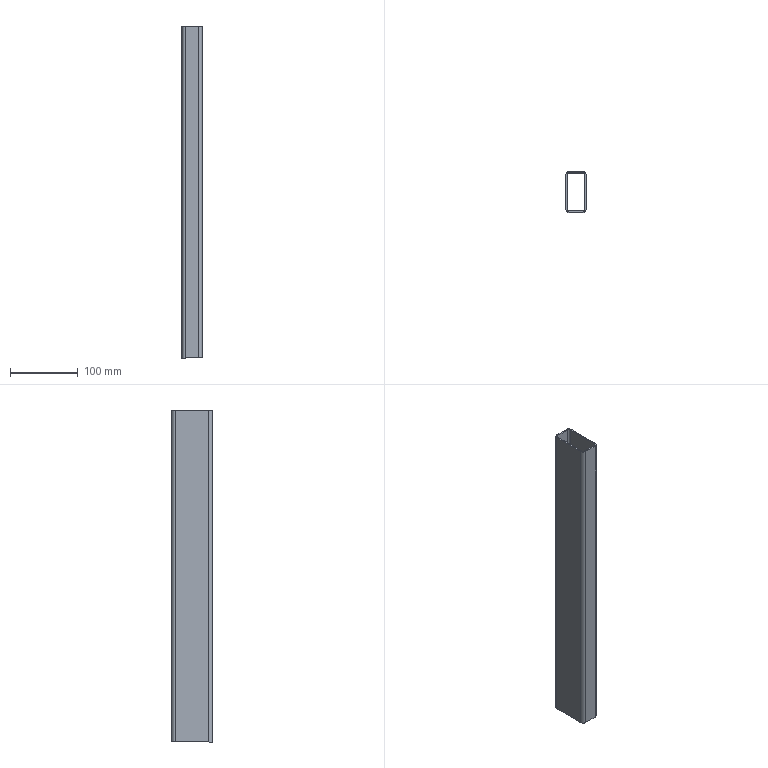Part | SolidWorks | features BaseBody 1 | 1 solid | 18 faces | box 30 x 60 x 490 mm | volume 161830 mm3 | plane 10 | cylinder 8 | commonest cylinder face diameters 6 x4 10 x4
STEP:
#1=CARTESIAN_POINT('',(10.,28.,490.));
#2=VERTEX_POINT('',#1);
#3=CARTESIAN_POINT('',(-10.,28.,490.));
#4=VERTEX_POINT('',#3);
#5=CARTESIAN_POINT('',(-5.,28.,490.));
#6=DIRECTION('',(-1.,0.,0.));
#7=VECTOR('',#6,1000.);
#8=LINE('',#5,#7);
#9=EDGE_CURVE('',#2,#4,#8,.T.);
#10=ORIENTED_EDGE('',*,*,#9,.F.);
#11=CARTESIAN_POINT('',(13.,25.,490.));
#12=VERTEX_POINT('',#11);
#13=CARTESIAN_POINT('',(10.,25.,490.));
#14=DIRECTION('',(0.,0.,1.));
#15=DIRECTION('',(-1.,0.,0.));
#16=AXIS2_PLACEMENT_3D('',#13,#14,#15);
#17=CIRCLE('',#16,3.);
#18=EDGE_CURVE('',#12,#2,#17,.T.);
#19=ORIENTED_EDGE('',*,*,#18,.F.);
#20=CARTESIAN_POINT('',(13.,-25.,490.));
#21=VERTEX_POINT('',#20);
#22=CARTESIAN_POINT('',(13.,12.5,490.));
#23=DIRECTION('',(0.,1.,0.));
#24=VECTOR('',#23,1000.);
#25=LINE('',#22,#24);
#26=EDGE_CURVE('',#21,#12,#25,.T.);
#27=ORIENTED_EDGE('',*,*,#26,.F.);
#28=CARTESIAN_POINT('',(10.,-28.,490.));
#29=VERTEX_POINT('',#28);
#30=CARTESIAN_POINT('',(10.,-25.,490.));
#31=DIRECTION('',(0.,0.,1.));
#32=DIRECTION('',(0.,1.,0.));
#33=AXIS2_PLACEMENT_3D('',#30,#31,#32);
#34=CIRCLE('',#33,3.);
#35=EDGE_CURVE('',#29,#21,#34,.T.);
#36=ORIENTED_EDGE('',*,*,#35,.F.);
#37=CARTESIAN_POINT('',(-10.,-28.,490.));
#38=VERTEX_POINT('',#37);
#39=CARTESIAN_POINT('',(5.,-28.,490.));
#40=DIRECTION('',(1.,0.,0.));
#41=VECTOR('',#40,1000.);
#42=LINE('',#39,#41);
#43=EDGE_CURVE('',#38,#29,#42,.T.);
#44=ORIENTED_EDGE('',*,*,#43,.F.);
#45=CARTESIAN_POINT('',(-13.,-25.,490.));
#46=VERTEX_POINT('',#45);
#47=CARTESIAN_POINT('',(-10.,-25.,490.));
#48=DIRECTION('',(0.,0.,1.));
#49=DIRECTION('',(1.,0.,0.));
#50=AXIS2_PLACEMENT_3D('',#47,#48,#49);
#51=CIRCLE('',#50,3.);
#52=EDGE_CURVE('',#46,#38,#51,.T.);
#53=ORIENTED_EDGE('',*,*,#52,.F.);
#54=CARTESIAN_POINT('',(-13.,25.,490.));
#55=VERTEX_POINT('',#54);
#56=CARTESIAN_POINT('',(-13.,-12.5,490.));
#57=DIRECTION('',(0.,-1.,0.));
#58=VECTOR('',#57,1000.);
#59=LINE('',#56,#58);
#60=EDGE_CURVE('',#55,#46,#59,.T.);
#61=ORIENTED_EDGE('',*,*,#60,.F.);
#62=CARTESIAN_POINT('',(-10.,25.,490.));
#63=DIRECTION('',(0.,0.,1.));
#64=DIRECTION('',(0.,-1.,0.));
#65=AXIS2_PLACEMENT_3D('',#62,#63,#64);
#66=CIRCLE('',#65,3.);
#67=EDGE_CURVE('',#4,#55,#66,.T.);
#68=ORIENTED_EDGE('',*,*,#67,.F.);
#69=EDGE_LOOP('',(#10,#19,#27,#36,#44,#53,#61,#68));
#70=FACE_BOUND('',#69,.T.);
#71=CARTESIAN_POINT('',(-15.,-25.,490.));
#72=VERTEX_POINT('',#71);
#73=CARTESIAN_POINT('',(-15.,25.,490.));
#74=VERTEX_POINT('',#73);
#75=CARTESIAN_POINT('',(-15.,-12.5,490.));
#76=DIRECTION('',(0.,1.,0.));
#77=VECTOR('',#76,1000.);
#78=LINE('',#75,#77);
#79=EDGE_CURVE('',#72,#74,#78,.T.);
#80=ORIENTED_EDGE('',*,*,#79,.F.);
#81=CARTESIAN_POINT('',(-10.,-30.,490.));
#82=VERTEX_POINT('',#81);
#83=CARTESIAN_POINT('',(-10.,-25.,490.));
#84=DIRECTION('',(0.,0.,-1.));
#85=DIRECTION('',(1.,0.,0.));
#86=AXIS2_PLACEMENT_3D('',#83,#84,#85);
#87=CIRCLE('',#86,5.);
#88=EDGE_CURVE('',#82,#72,#87,.T.);
#89=ORIENTED_EDGE('',*,*,#88,.F.);
#90=CARTESIAN_POINT('',(10.,-30.,490.));
#91=VERTEX_POINT('',#90);
#92=CARTESIAN_POINT('',(5.,-30.,490.));
#93=DIRECTION('',(-1.,0.,0.));
#94=VECTOR('',#93,1000.);
#95=LINE('',#92,#94);
#96=EDGE_CURVE('',#91,#82,#95,.T.);
#97=ORIENTED_EDGE('',*,*,#96,.F.);
#98=CARTESIAN_POINT('',(15.,-25.,490.));
#99=VERTEX_POINT('',#98);
#100=CARTESIAN_POINT('',(10.,-25.,490.));
#101=DIRECTION('',(0.,0.,-1.));
#102=DIRECTION('',(0.,1.,0.));
#103=AXIS2_PLACEMENT_3D('',#100,#101,#102);
#104=CIRCLE('',#103,5.);
#105=EDGE_CURVE('',#99,#91,#104,.T.);
#106=ORIENTED_EDGE('',*,*,#105,.F.);
#107=CARTESIAN_POINT('',(15.,25.,490.));
#108=VERTEX_POINT('',#107);
#109=CARTESIAN_POINT('',(15.,12.5,490.));
#110=DIRECTION('',(0.,-1.,0.));
#111=VECTOR('',#110,1000.);
#112=LINE('',#109,#111);
#113=EDGE_CURVE('',#108,#99,#112,.T.);
#114=ORIENTED_EDGE('',*,*,#113,.F.);
#115=CARTESIAN_POINT('',(10.,30.,490.));
#116=VERTEX_POINT('',#115);
#117=CARTESIAN_POINT('',(10.,25.,490.));
#118=DIRECTION('',(0.,0.,-1.));
#119=DIRECTION('',(-1.,0.,0.));
#120=AXIS2_PLACEMENT_3D('',#117,#118,#119);
#121=CIRCLE('',#120,5.);
#122=EDGE_CURVE('',#116,#108,#121,.T.);
#123=ORIENTED_EDGE('',*,*,#122,.F.);
#124=CARTESIAN_POINT('',(-10.,30.,490.));
#125=VERTEX_POINT('',#124);
#126=CARTESIAN_POINT('',(-5.,30.,490.));
#127=DIRECTION('',(1.,0.,0.));
#128=VECTOR('',#127,1000.);
#129=LINE('',#126,#128);
#130=EDGE_CURVE('',#125,#116,#129,.T.);
#131=ORIENTED_EDGE('',*,*,#130,.F.);
#132=CARTESIAN_POINT('',(-10.,25.,490.));
#133=DIRECTION('',(0.,0.,-1.));
#134=DIRECTION('',(0.,-1.,0.));
#135=AXIS2_PLACEMENT_3D('',#132,#133,#134);
#136=CIRCLE('',#135,5.);
#137=EDGE_CURVE('',#74,#125,#136,.T.);
#138=ORIENTED_EDGE('',*,*,#137,.F.);
#139=EDGE_LOOP('',(#80,#89,#97,#106,#114,#123,#131,#138));
#140=FACE_OUTER_BOUND('',#139,.T.);
#141=CARTESIAN_POINT('',(0.,0.,490.));
#142=DIRECTION('',(0.,0.,1.));
#143=DIRECTION('',(1.,0.,0.));
#144=AXIS2_PLACEMENT_3D('',#141,#142,#143);
#145=PLANE('',#144);
#146=ADVANCED_FACE('',(#70,#140),#145,.T.);
#147=CARTESIAN_POINT('',(10.,28.,0.));
#148=VERTEX_POINT('',#147);
#149=CARTESIAN_POINT('',(-10.,28.,0.));
#150=VERTEX_POINT('',#149);
#151=CARTESIAN_POINT('',(-5.,28.,0.));
#152=DIRECTION('',(-1.,0.,0.));
#153=VECTOR('',#152,1000.);
#154=LINE('',#151,#153);
#155=EDGE_CURVE('',#148,#150,#154,.T.);
#156=ORIENTED_EDGE('',*,*,#155,.T.);
#157=CARTESIAN_POINT('',(-13.,25.,0.));
#158=VERTEX_POINT('',#157);
#159=CARTESIAN_POINT('',(-10.,25.,0.));
#160=DIRECTION('',(0.,0.,1.));
#161=DIRECTION('',(0.,-1.,0.));
#162=AXIS2_PLACEMENT_3D('',#159,#160,#161);
#163=CIRCLE('',#162,3.);
#164=EDGE_CURVE('',#150,#158,#163,.T.);
#165=ORIENTED_EDGE('',*,*,#164,.T.);
#166=CARTESIAN_POINT('',(-13.,-25.,0.));
#167=VERTEX_POINT('',#166);
#168=CARTESIAN_POINT('',(-13.,-12.5,0.));
#169=DIRECTION('',(0.,-1.,0.));
#170=VECTOR('',#169,1000.);
#171=LINE('',#168,#170);
#172=EDGE_CURVE('',#158,#167,#171,.T.);
#173=ORIENTED_EDGE('',*,*,#172,.T.);
#174=CARTESIAN_POINT('',(-10.,-28.,0.));
#175=VERTEX_POINT('',#174);
#176=CARTESIAN_POINT('',(-10.,-25.,0.));
#177=DIRECTION('',(0.,0.,1.));
#178=DIRECTION('',(1.,0.,0.));
#179=AXIS2_PLACEMENT_3D('',#176,#177,#178);
#180=CIRCLE('',#179,3.);
#181=EDGE_CURVE('',#167,#175,#180,.T.);
#182=ORIENTED_EDGE('',*,*,#181,.T.);
#183=CARTESIAN_POINT('',(10.,-28.,0.));
#184=VERTEX_POINT('',#183);
#185=CARTESIAN_POINT('',(5.,-28.,0.));
#186=DIRECTION('',(1.,0.,0.));
#187=VECTOR('',#186,1000.);
#188=LINE('',#185,#187);
#189=EDGE_CURVE('',#175,#184,#188,.T.);
#190=ORIENTED_EDGE('',*,*,#189,.T.);
#191=CARTESIAN_POINT('',(13.,-25.,0.));
#192=VERTEX_POINT('',#191);
#193=CARTESIAN_POINT('',(10.,-25.,0.));
#194=DIRECTION('',(0.,0.,1.));
#195=DIRECTION('',(0.,1.,0.));
#196=AXIS2_PLACEMENT_3D('',#193,#194,#195);
#197=CIRCLE('',#196,3.);
#198=EDGE_CURVE('',#184,#192,#197,.T.);
#199=ORIENTED_EDGE('',*,*,#198,.T.);
#200=CARTESIAN_POINT('',(13.,25.,0.));
#201=VERTEX_POINT('',#200);
#202=CARTESIAN_POINT('',(13.,12.5,0.));
#203=DIRECTION('',(0.,1.,0.));
#204=VECTOR('',#203,1000.);
#205=LINE('',#202,#204);
#206=EDGE_CURVE('',#192,#201,#205,.T.);
#207=ORIENTED_EDGE('',*,*,#206,.T.);
#208=CARTESIAN_POINT('',(10.,25.,0.));
#209=DIRECTION('',(0.,0.,1.));
#210=DIRECTION('',(-1.,0.,0.));
#211=AXIS2_PLACEMENT_3D('',#208,#209,#210);
#212=CIRCLE('',#211,3.);
#213=EDGE_CURVE('',#201,#148,#212,.T.);
#214=ORIENTED_EDGE('',*,*,#213,.T.);
#215=EDGE_LOOP('',(#156,#165,#173,#182,#190,#199,#207,#214));
#216=FACE_BOUND('',#215,.T.);
#217=CARTESIAN_POINT('',(-15.,-25.,0.));
#218=VERTEX_POINT('',#217);
#219=CARTESIAN_POINT('',(-15.,25.,0.));
#220=VERTEX_POINT('',#219);
#221=CARTESIAN_POINT('',(-15.,-12.5,0.));
#222=DIRECTION('',(0.,1.,0.));
#223=VECTOR('',#222,1000.);
#224=LINE('',#221,#223);
#225=EDGE_CURVE('',#218,#220,#224,.T.);
#226=ORIENTED_EDGE('',*,*,#225,.T.);
#227=CARTESIAN_POINT('',(-10.,30.,0.));
#228=VERTEX_POINT('',#227);
#229=CARTESIAN_POINT('',(-10.,25.,0.));
#230=DIRECTION('',(0.,0.,-1.));
#231=DIRECTION('',(0.,-1.,0.));
#232=AXIS2_PLACEMENT_3D('',#229,#230,#231);
#233=CIRCLE('',#232,5.);
#234=EDGE_CURVE('',#220,#228,#233,.T.);
#235=ORIENTED_EDGE('',*,*,#234,.T.);
#236=CARTESIAN_POINT('',(10.,30.,0.));
#237=VERTEX_POINT('',#236);
#238=CARTESIAN_POINT('',(-5.,30.,0.));
#239=DIRECTION('',(1.,0.,0.));
#240=VECTOR('',#239,1000.);
#241=LINE('',#238,#240);
#242=EDGE_CURVE('',#228,#237,#241,.T.);
#243=ORIENTED_EDGE('',*,*,#242,.T.);
#244=CARTESIAN_POINT('',(15.,25.,0.));
#245=VERTEX_POINT('',#244);
#246=CARTESIAN_POINT('',(10.,25.,0.));
#247=DIRECTION('',(0.,0.,-1.));
#248=DIRECTION('',(-1.,0.,0.));
#249=AXIS2_PLACEMENT_3D('',#246,#247,#248);
#250=CIRCLE('',#249,5.);
#251=EDGE_CURVE('',#237,#245,#250,.T.);
#252=ORIENTED_EDGE('',*,*,#251,.T.);
#253=CARTESIAN_POINT('',(15.,-25.,0.));
#254=VERTEX_POINT('',#253);
#255=CARTESIAN_POINT('',(15.,12.5,0.));
#256=DIRECTION('',(0.,-1.,0.));
#257=VECTOR('',#256,1000.);
#258=LINE('',#255,#257);
#259=EDGE_CURVE('',#245,#254,#258,.T.);
#260=ORIENTED_EDGE('',*,*,#259,.T.);
#261=CARTESIAN_POINT('',(10.,-30.,0.));
#262=VERTEX_POINT('',#261);
#263=CARTESIAN_POINT('',(10.,-25.,0.));
#264=DIRECTION('',(0.,0.,-1.));
#265=DIRECTION('',(0.,1.,0.));
#266=AXIS2_PLACEMENT_3D('',#263,#264,#265);
#267=CIRCLE('',#266,5.);
#268=EDGE_CURVE('',#254,#262,#267,.T.);
#269=ORIENTED_EDGE('',*,*,#268,.T.);
#270=CARTESIAN_POINT('',(-10.,-30.,0.));
#271=VERTEX_POINT('',#270);
#272=CARTESIAN_POINT('',(5.,-30.,0.));
#273=DIRECTION('',(-1.,0.,0.));
#274=VECTOR('',#273,1000.);
#275=LINE('',#272,#274);
#276=EDGE_CURVE('',#262,#271,#275,.T.);
#277=ORIENTED_EDGE('',*,*,#276,.T.);
#278=CARTESIAN_POINT('',(-10.,-25.,0.));
#279=DIRECTION('',(0.,0.,-1.));
#280=DIRECTION('',(1.,0.,0.));
#281=AXIS2_PLACEMENT_3D('',#278,#279,#280);
#282=CIRCLE('',#281,5.);
#283=EDGE_CURVE('',#271,#218,#282,.T.);
#284=ORIENTED_EDGE('',*,*,#283,.T.);
#285=EDGE_LOOP('',(#226,#235,#243,#252,#260,#269,#277,#284));
#286=FACE_OUTER_BOUND('',#285,.T.);
#287=CARTESIAN_POINT('',(0.,0.,0.));
#288=DIRECTION('',(0.,0.,1.));
#289=DIRECTION('',(1.,0.,0.));
#290=AXIS2_PLACEMENT_3D('',#287,#288,#289);
#291=PLANE('',#290);
#292=ADVANCED_FACE('',(#216,#286),#291,.F.);
#293=ORIENTED_EDGE('',*,*,#122,.T.);
#294=CARTESIAN_POINT('',(15.,25.,0.));
#295=DIRECTION('',(0.,0.,1.));
#296=VECTOR('',#295,1000.);
#297=LINE('',#294,#296);
#298=EDGE_CURVE('',#245,#108,#297,.T.);
#299=ORIENTED_EDGE('',*,*,#298,.F.);
#300=ORIENTED_EDGE('',*,*,#251,.F.);
#301=CARTESIAN_POINT('',(10.,30.,0.));
#302=DIRECTION('',(0.,0.,1.));
#303=VECTOR('',#302,1000.);
#304=LINE('',#301,#303);
#305=EDGE_CURVE('',#237,#116,#304,.T.);
#306=ORIENTED_EDGE('',*,*,#305,.T.);
#307=EDGE_LOOP('',(#293,#299,#300,#306));
#308=FACE_OUTER_BOUND('',#307,.T.);
#309=CARTESIAN_POINT('',(10.,25.,0.));
#310=DIRECTION('',(0.,0.,1.));
#311=DIRECTION('',(-1.,0.,0.));
#312=AXIS2_PLACEMENT_3D('',#309,#310,#311);
#313=CYLINDRICAL_SURFACE('',#312,5.);
#314=ADVANCED_FACE('',(#308),#313,.T.);
#315=ORIENTED_EDGE('',*,*,#130,.T.);
#316=ORIENTED_EDGE('',*,*,#305,.F.);
#317=ORIENTED_EDGE('',*,*,#242,.F.);
#318=CARTESIAN_POINT('',(-10.,30.,0.));
#319=DIRECTION('',(0.,0.,1.));
#320=VECTOR('',#319,1000.);
#321=LINE('',#318,#320);
#322=EDGE_CURVE('',#228,#125,#321,.T.);
#323=ORIENTED_EDGE('',*,*,#322,.T.);
#324=EDGE_LOOP('',(#315,#316,#317,#323));
#325=FACE_OUTER_BOUND('',#324,.T.);
#326=CARTESIAN_POINT('',(-10.,30.,0.));
#327=DIRECTION('',(0.,1.,0.));
#328=DIRECTION('',(1.,0.,0.));
#329=AXIS2_PLACEMENT_3D('',#326,#327,#328);
#330=PLANE('',#329);
#331=ADVANCED_FACE('',(#325),#330,.T.);
#332=ORIENTED_EDGE('',*,*,#137,.T.);
#333=ORIENTED_EDGE('',*,*,#322,.F.);
#334=ORIENTED_EDGE('',*,*,#234,.F.);
#335=CARTESIAN_POINT('',(-15.,25.,0.));
#336=DIRECTION('',(0.,0.,1.));
#337=VECTOR('',#336,1000.);
#338=LINE('',#335,#337);
#339=EDGE_CURVE('',#220,#74,#338,.T.);
#340=ORIENTED_EDGE('',*,*,#339,.T.);
#341=EDGE_LOOP('',(#332,#333,#334,#340));
#342=FACE_OUTER_BOUND('',#341,.T.);
#343=CARTESIAN_POINT('',(-10.,25.,0.));
#344=DIRECTION('',(0.,0.,1.));
#345=DIRECTION('',(0.,-1.,0.));
#346=AXIS2_PLACEMENT_3D('',#343,#344,#345);
#347=CYLINDRICAL_SURFACE('',#346,5.);
#348=ADVANCED_FACE('',(#342),#347,.T.);
#349=ORIENTED_EDGE('',*,*,#79,.T.);
#350=ORIENTED_EDGE('',*,*,#339,.F.);
#351=ORIENTED_EDGE('',*,*,#225,.F.);
#352=CARTESIAN_POINT('',(-15.,-25.,0.));
#353=DIRECTION('',(0.,0.,1.));
#354=VECTOR('',#353,1000.);
#355=LINE('',#352,#354);
#356=EDGE_CURVE('',#218,#72,#355,.T.);
#357=ORIENTED_EDGE('',*,*,#356,.T.);
#358=EDGE_LOOP('',(#349,#350,#351,#357));
#359=FACE_OUTER_BOUND('',#358,.T.);
#360=CARTESIAN_POINT('',(-15.,-25.,0.));
#361=DIRECTION('',(-1.,0.,0.));
#362=DIRECTION('',(0.,1.,0.));
#363=AXIS2_PLACEMENT_3D('',#360,#361,#362);
#364=PLANE('',#363);
#365=ADVANCED_FACE('',(#359),#364,.T.);
#366=ORIENTED_EDGE('',*,*,#67,.T.);
#367=CARTESIAN_POINT('',(-13.,25.,0.));
#368=DIRECTION('',(0.,0.,1.));
#369=VECTOR('',#368,1000.);
#370=LINE('',#367,#369);
#371=EDGE_CURVE('',#158,#55,#370,.T.);
#372=ORIENTED_EDGE('',*,*,#371,.F.);
#373=ORIENTED_EDGE('',*,*,#164,.F.);
#374=CARTESIAN_POINT('',(-10.,28.,0.));
#375=DIRECTION('',(0.,0.,1.));
#376=VECTOR('',#375,1000.);
#377=LINE('',#374,#376);
#378=EDGE_CURVE('',#150,#4,#377,.T.);
#379=ORIENTED_EDGE('',*,*,#378,.T.);
#380=EDGE_LOOP('',(#366,#372,#373,#379));
#381=FACE_OUTER_BOUND('',#380,.T.);
#382=CARTESIAN_POINT('',(-10.,25.,0.));
#383=DIRECTION('',(0.,0.,1.));
#384=DIRECTION('',(0.,-1.,0.));
#385=AXIS2_PLACEMENT_3D('',#382,#383,#384);
#386=CYLINDRICAL_SURFACE('',#385,3.);
#387=ADVANCED_FACE('',(#381),#386,.F.);
#388=ORIENTED_EDGE('',*,*,#60,.T.);
#389=CARTESIAN_POINT('',(-13.,-25.,0.));
#390=DIRECTION('',(0.,0.,1.));
#391=VECTOR('',#390,1000.);
#392=LINE('',#389,#391);
#393=EDGE_CURVE('',#167,#46,#392,.T.);
#394=ORIENTED_EDGE('',*,*,#393,.F.);
#395=ORIENTED_EDGE('',*,*,#172,.F.);
#396=ORIENTED_EDGE('',*,*,#371,.T.);
#397=EDGE_LOOP('',(#388,#394,#395,#396));
#398=FACE_OUTER_BOUND('',#397,.T.);
#399=CARTESIAN_POINT('',(-13.,-25.,0.));
#400=DIRECTION('',(-1.,0.,0.));
#401=DIRECTION('',(0.,1.,0.));
#402=AXIS2_PLACEMENT_3D('',#399,#400,#401);
#403=PLANE('',#402);
#404=ADVANCED_FACE('',(#398),#403,.F.);
#405=ORIENTED_EDGE('',*,*,#52,.T.);
#406=CARTESIAN_POINT('',(-10.,-28.,0.));
#407=DIRECTION('',(0.,0.,1.));
#408=VECTOR('',#407,1000.);
#409=LINE('',#406,#408);
#410=EDGE_CURVE('',#175,#38,#409,.T.);
#411=ORIENTED_EDGE('',*,*,#410,.F.);
#412=ORIENTED_EDGE('',*,*,#181,.F.);
#413=ORIENTED_EDGE('',*,*,#393,.T.);
#414=EDGE_LOOP('',(#405,#411,#412,#413));
#415=FACE_OUTER_BOUND('',#414,.T.);
#416=CARTESIAN_POINT('',(-10.,-25.,0.));
#417=DIRECTION('',(0.,0.,1.));
#418=DIRECTION('',(1.,0.,0.));
#419=AXIS2_PLACEMENT_3D('',#416,#417,#418);
#420=CYLINDRICAL_SURFACE('',#419,3.);
#421=ADVANCED_FACE('',(#415),#420,.F.);
#422=ORIENTED_EDGE('',*,*,#9,.T.);
#423=ORIENTED_EDGE('',*,*,#378,.F.);
#424=ORIENTED_EDGE('',*,*,#155,.F.);
#425=CARTESIAN_POINT('',(10.,28.,0.));
#426=DIRECTION('',(0.,0.,1.));
#427=VECTOR('',#426,1000.);
#428=LINE('',#425,#427);
#429=EDGE_CURVE('',#148,#2,#428,.T.);
#430=ORIENTED_EDGE('',*,*,#429,.T.);
#431=EDGE_LOOP('',(#422,#423,#424,#430));
#432=FACE_OUTER_BOUND('',#431,.T.);
#433=CARTESIAN_POINT('',(-10.,28.,0.));
#434=DIRECTION('',(0.,1.,0.));
#435=DIRECTION('',(1.,0.,0.));
#436=AXIS2_PLACEMENT_3D('',#433,#434,#435);
#437=PLANE('',#436);
#438=ADVANCED_FACE('',(#432),#437,.F.);
#439=ORIENTED_EDGE('',*,*,#88,.T.);
#440=ORIENTED_EDGE('',*,*,#356,.F.);
#441=ORIENTED_EDGE('',*,*,#283,.F.);
#442=CARTESIAN_POINT('',(-10.,-30.,0.));
#443=DIRECTION('',(0.,0.,1.));
#444=VECTOR('',#443,1000.);
#445=LINE('',#442,#444);
#446=EDGE_CURVE('',#271,#82,#445,.T.);
#447=ORIENTED_EDGE('',*,*,#446,.T.);
#448=EDGE_LOOP('',(#439,#440,#441,#447));
#449=FACE_OUTER_BOUND('',#448,.T.);
#450=CARTESIAN_POINT('',(-10.,-25.,0.));
#451=DIRECTION('',(0.,0.,1.));
#452=DIRECTION('',(1.,0.,0.));
#453=AXIS2_PLACEMENT_3D('',#450,#451,#452);
#454=CYLINDRICAL_SURFACE('',#453,5.);
#455=ADVANCED_FACE('',(#449),#454,.T.);
#456=ORIENTED_EDGE('',*,*,#96,.T.);
#457=ORIENTED_EDGE('',*,*,#446,.F.);
#458=ORIENTED_EDGE('',*,*,#276,.F.);
#459=CARTESIAN_POINT('',(10.,-30.,0.));
#460=DIRECTION('',(0.,0.,1.));
#461=VECTOR('',#460,1000.);
#462=LINE('',#459,#461);
#463=EDGE_CURVE('',#262,#91,#462,.T.);
#464=ORIENTED_EDGE('',*,*,#463,.T.);
#465=EDGE_LOOP('',(#456,#457,#458,#464));
#466=FACE_OUTER_BOUND('',#465,.T.);
#467=CARTESIAN_POINT('',(10.,-30.,0.));
#468=DIRECTION('',(0.,-1.,0.));
#469=DIRECTION('',(0.,0.,-1.));
#470=AXIS2_PLACEMENT_3D('',#467,#468,#469);
#471=PLANE('',#470);
#472=ADVANCED_FACE('',(#466),#471,.T.);
#473=ORIENTED_EDGE('',*,*,#105,.T.);
#474=ORIENTED_EDGE('',*,*,#463,.F.);
#475=ORIENTED_EDGE('',*,*,#268,.F.);
#476=CARTESIAN_POINT('',(15.,-25.,0.));
#477=DIRECTION('',(0.,0.,1.));
#478=VECTOR('',#477,1000.);
#479=LINE('',#476,#478);
#480=EDGE_CURVE('',#254,#99,#479,.T.);
#481=ORIENTED_EDGE('',*,*,#480,.T.);
#482=EDGE_LOOP('',(#473,#474,#475,#481));
#483=FACE_OUTER_BOUND('',#482,.T.);
#484=CARTESIAN_POINT('',(10.,-25.,0.));
#485=DIRECTION('',(0.,0.,1.));
#486=DIRECTION('',(0.,1.,0.));
#487=AXIS2_PLACEMENT_3D('',#484,#485,#486);
#488=CYLINDRICAL_SURFACE('',#487,5.);
#489=ADVANCED_FACE('',(#483),#488,.T.);
#490=ORIENTED_EDGE('',*,*,#113,.T.);
#491=ORIENTED_EDGE('',*,*,#480,.F.);
#492=ORIENTED_EDGE('',*,*,#259,.F.);
#493=ORIENTED_EDGE('',*,*,#298,.T.);
#494=EDGE_LOOP('',(#490,#491,#492,#493));
#495=FACE_OUTER_BOUND('',#494,.T.);
#496=CARTESIAN_POINT('',(15.,25.,0.));
#497=DIRECTION('',(1.,0.,0.));
#498=DIRECTION('',(0.,1.,0.));
#499=AXIS2_PLACEMENT_3D('',#496,#497,#498);
#500=PLANE('',#499);
#501=ADVANCED_FACE('',(#495),#500,.T.);
#502=ORIENTED_EDGE('',*,*,#18,.T.);
#503=ORIENTED_EDGE('',*,*,#429,.F.);
#504=ORIENTED_EDGE('',*,*,#213,.F.);
#505=CARTESIAN_POINT('',(13.,25.,0.));
#506=DIRECTION('',(0.,0.,1.));
#507=VECTOR('',#506,1000.);
#508=LINE('',#505,#507);
#509=EDGE_CURVE('',#201,#12,#508,.T.);
#510=ORIENTED_EDGE('',*,*,#509,.T.);
#511=EDGE_LOOP('',(#502,#503,#504,#510));
#512=FACE_OUTER_BOUND('',#511,.T.);
#513=CARTESIAN_POINT('',(10.,25.,0.));
#514=DIRECTION('',(0.,0.,1.));
#515=DIRECTION('',(-1.,0.,0.));
#516=AXIS2_PLACEMENT_3D('',#513,#514,#515);
#517=CYLINDRICAL_SURFACE('',#516,3.);
#518=ADVANCED_FACE('',(#512),#517,.F.);
#519=ORIENTED_EDGE('',*,*,#26,.T.);
#520=ORIENTED_EDGE('',*,*,#509,.F.);
#521=ORIENTED_EDGE('',*,*,#206,.F.);
#522=CARTESIAN_POINT('',(13.,-25.,0.));
#523=DIRECTION('',(0.,0.,1.));
#524=VECTOR('',#523,1000.);
#525=LINE('',#522,#524);
#526=EDGE_CURVE('',#192,#21,#525,.T.);
#527=ORIENTED_EDGE('',*,*,#526,.T.);
#528=EDGE_LOOP('',(#519,#520,#521,#527));
#529=FACE_OUTER_BOUND('',#528,.T.);
#530=CARTESIAN_POINT('',(13.,25.,0.));
#531=DIRECTION('',(1.,0.,0.));
#532=DIRECTION('',(0.,1.,0.));
#533=AXIS2_PLACEMENT_3D('',#530,#531,#532);
#534=PLANE('',#533);
#535=ADVANCED_FACE('',(#529),#534,.F.);
#536=ORIENTED_EDGE('',*,*,#35,.T.);
#537=ORIENTED_EDGE('',*,*,#526,.F.);
#538=ORIENTED_EDGE('',*,*,#198,.F.);
#539=CARTESIAN_POINT('',(10.,-28.,0.));
#540=DIRECTION('',(0.,0.,1.));
#541=VECTOR('',#540,1000.);
#542=LINE('',#539,#541);
#543=EDGE_CURVE('',#184,#29,#542,.T.);
#544=ORIENTED_EDGE('',*,*,#543,.T.);
#545=EDGE_LOOP('',(#536,#537,#538,#544));
#546=FACE_OUTER_BOUND('',#545,.T.);
#547=CARTESIAN_POINT('',(10.,-25.,0.));
#548=DIRECTION('',(0.,0.,1.));
#549=DIRECTION('',(0.,1.,0.));
#550=AXIS2_PLACEMENT_3D('',#547,#548,#549);
#551=CYLINDRICAL_SURFACE('',#550,3.);
#552=ADVANCED_FACE('',(#546),#551,.F.);
#553=ORIENTED_EDGE('',*,*,#43,.T.);
#554=ORIENTED_EDGE('',*,*,#543,.F.);
#555=ORIENTED_EDGE('',*,*,#189,.F.);
#556=ORIENTED_EDGE('',*,*,#410,.T.);
#557=EDGE_LOOP('',(#553,#554,#555,#556));
#558=FACE_OUTER_BOUND('',#557,.T.);
#559=CARTESIAN_POINT('',(10.,-28.,0.));
#560=DIRECTION('',(0.,-1.,0.));
#561=DIRECTION('',(0.,0.,-1.));
#562=AXIS2_PLACEMENT_3D('',#559,#560,#561);
#563=PLANE('',#562);
#564=ADVANCED_FACE('',(#558),#563,.F.);
#565=CLOSED_SHELL('',(#146,#292,#314,#331,#348,#365,#387,#404,#421,#438,#455,#472,#489,#501,#518,#535,#552,#564));
#566=MANIFOLD_SOLID_BREP('',#565);
#567=CARTESIAN_POINT('',(0.,0.,0.));
#568=DIRECTION('',(0.,0.,1.));
#569=DIRECTION('',(1.,0.,0.));
#570=AXIS2_PLACEMENT_3D('',#567,#568,#569);
#571=(LENGTH_UNIT()NAMED_UNIT(*)SI_UNIT(.MILLI.,.METRE.));
#572=UNCERTAINTY_MEASURE_WITH_UNIT(LENGTH_MEASURE(0.00001),#571,'','');
#573=(NAMED_UNIT(*)PLANE_ANGLE_UNIT()SI_UNIT($,.RADIAN.));
#574=(NAMED_UNIT(*)SI_UNIT($,.STERADIAN.)SOLID_ANGLE_UNIT());
#575=(GEOMETRIC_REPRESENTATION_CONTEXT(3)GLOBAL_UNCERTAINTY_ASSIGNED_CONTEXT((#572))GLOBAL_UNIT_ASSIGNED_CONTEXT((#571,#573,#574))REPRESENTATION_CONTEXT('',''));
#576=ADVANCED_BREP_SHAPE_REPRESENTATION('',(#566,#570),#575);